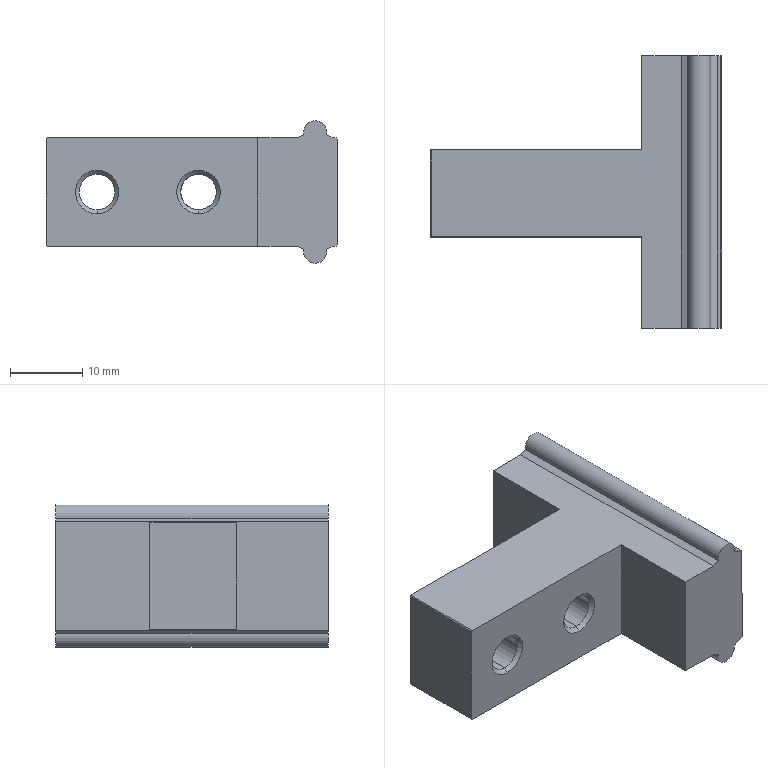Part | SolidWorks | features BaseBody 1 | 1 solid | 35 faces | box 40.2 x 37.6 x 19.68 mm | volume 11497 mm3 | plane 20 | cone 8 | cylinder 7 | commonest cylinder face diameters 4.917 x4 3.18 x3
STEP:
#1=CARTESIAN_POINT('',(-75.9,-11.,-9.84));
#2=VERTEX_POINT('',#1);
#3=CARTESIAN_POINT('',(-77.453,-11.,-7.911));
#4=VERTEX_POINT('',#3);
#5=CARTESIAN_POINT('',(-75.9,-11.,-8.25));
#6=DIRECTION('',(0.,1.,0.));
#7=DIRECTION('',(0.,0.,-1.));
#8=AXIS2_PLACEMENT_3D('',#5,#6,#7);
#9=CIRCLE('',#8,1.59);
#10=EDGE_CURVE('',#2,#4,#9,.T.);
#11=ORIENTED_EDGE('',*,*,#10,.F.);
#12=CARTESIAN_POINT('',(-75.9,-48.6,-9.84));
#13=VERTEX_POINT('',#12);
#14=CARTESIAN_POINT('',(-75.9,-48.6,-9.84));
#15=DIRECTION('',(0.,-1.,0.));
#16=VECTOR('',#15,1000.);
#17=LINE('',#14,#16);
#18=EDGE_CURVE('',#2,#13,#17,.T.);
#19=ORIENTED_EDGE('',*,*,#18,.T.);
#20=CARTESIAN_POINT('',(-77.453,-48.6,-7.911));
#21=VERTEX_POINT('',#20);
#22=CARTESIAN_POINT('',(-75.9,-48.6,-8.25));
#23=DIRECTION('',(0.,1.,0.));
#24=DIRECTION('',(0.,0.,-1.));
#25=AXIS2_PLACEMENT_3D('',#22,#23,#24);
#26=CIRCLE('',#25,1.59);
#27=EDGE_CURVE('',#13,#21,#26,.T.);
#28=ORIENTED_EDGE('',*,*,#27,.T.);
#29=CARTESIAN_POINT('',(-77.453,-48.6,-7.911));
#30=DIRECTION('',(0.,1.,0.));
#31=VECTOR('',#30,1000.);
#32=LINE('',#29,#31);
#33=EDGE_CURVE('',#21,#4,#32,.T.);
#34=ORIENTED_EDGE('',*,*,#33,.T.);
#35=EDGE_LOOP('',(#11,#19,#28,#34));
#36=FACE_OUTER_BOUND('',#35,.T.);
#37=CARTESIAN_POINT('',(-75.9,-48.6,-8.25));
#38=DIRECTION('',(0.,-1.,0.));
#39=DIRECTION('',(0.,0.,-1.));
#40=AXIS2_PLACEMENT_3D('',#37,#38,#39);
#41=CYLINDRICAL_SURFACE('',#40,1.59);
#42=ADVANCED_FACE('',(#36),#41,.T.);
#43=CARTESIAN_POINT('',(-92.,-35.459,2.458));
#44=VERTEX_POINT('',#43);
#45=CARTESIAN_POINT('',(-92.,-35.459,-2.458));
#46=VERTEX_POINT('',#45);
#47=CARTESIAN_POINT('',(-92.,-35.459,0.));
#48=DIRECTION('',(0.,-1.,0.));
#49=DIRECTION('',(0.,0.,-1.));
#50=AXIS2_PLACEMENT_3D('',#47,#48,#49);
#51=CIRCLE('',#50,2.458);
#52=EDGE_CURVE('',#44,#46,#51,.T.);
#53=ORIENTED_EDGE('',*,*,#52,.F.);
#54=CARTESIAN_POINT('',(-92.,-36.,3.));
#55=VERTEX_POINT('',#54);
#56=CARTESIAN_POINT('',(-92.,-36.,3.));
#57=DIRECTION('',(0.,-0.7071,0.7071));
#58=VECTOR('',#57,1000.);
#59=LINE('',#56,#58);
#60=EDGE_CURVE('',#44,#55,#59,.T.);
#61=ORIENTED_EDGE('',*,*,#60,.T.);
#62=CARTESIAN_POINT('',(-92.,-36.,-3.));
#63=VERTEX_POINT('',#62);
#64=CARTESIAN_POINT('',(-92.,-36.,0.));
#65=DIRECTION('',(0.,-1.,0.));
#66=DIRECTION('',(0.,0.,-1.));
#67=AXIS2_PLACEMENT_3D('',#64,#65,#66);
#68=CIRCLE('',#67,3.);
#69=EDGE_CURVE('',#55,#63,#68,.T.);
#70=ORIENTED_EDGE('',*,*,#69,.T.);
#71=CARTESIAN_POINT('',(-92.,-36.,-3.));
#72=DIRECTION('',(0.,-0.7071,-0.7071));
#73=VECTOR('',#72,1000.);
#74=LINE('',#71,#73);
#75=EDGE_CURVE('',#46,#63,#74,.T.);
#76=ORIENTED_EDGE('',*,*,#75,.F.);
#77=EDGE_LOOP('',(#53,#61,#70,#76));
#78=FACE_OUTER_BOUND('',#77,.T.);
#79=CARTESIAN_POINT('',(-92.,-36.,0.));
#80=DIRECTION('',(0.,-1.,0.));
#81=DIRECTION('',(0.,0.,-1.));
#82=AXIS2_PLACEMENT_3D('',#79,#80,#81);
#83=CONICAL_SURFACE('',#82,3.,0.7854);
#84=ADVANCED_FACE('',(#78),#83,.F.);
#85=CARTESIAN_POINT('',(-106.,-35.459,2.458));
#86=VERTEX_POINT('',#85);
#87=CARTESIAN_POINT('',(-106.,-35.459,-2.458));
#88=VERTEX_POINT('',#87);
#89=CARTESIAN_POINT('',(-106.,-35.459,0.));
#90=DIRECTION('',(0.,-1.,0.));
#91=DIRECTION('',(0.,0.,-1.));
#92=AXIS2_PLACEMENT_3D('',#89,#90,#91);
#93=CIRCLE('',#92,2.458);
#94=EDGE_CURVE('',#86,#88,#93,.T.);
#95=ORIENTED_EDGE('',*,*,#94,.F.);
#96=CARTESIAN_POINT('',(-106.,-36.,3.));
#97=VERTEX_POINT('',#96);
#98=CARTESIAN_POINT('',(-106.,-36.,3.));
#99=DIRECTION('',(0.,-0.7071,0.7071));
#100=VECTOR('',#99,1000.);
#101=LINE('',#98,#100);
#102=EDGE_CURVE('',#86,#97,#101,.T.);
#103=ORIENTED_EDGE('',*,*,#102,.T.);
#104=CARTESIAN_POINT('',(-106.,-36.,-3.));
#105=VERTEX_POINT('',#104);
#106=CARTESIAN_POINT('',(-106.,-36.,0.));
#107=DIRECTION('',(0.,-1.,0.));
#108=DIRECTION('',(0.,0.,-1.));
#109=AXIS2_PLACEMENT_3D('',#106,#107,#108);
#110=CIRCLE('',#109,3.);
#111=EDGE_CURVE('',#97,#105,#110,.T.);
#112=ORIENTED_EDGE('',*,*,#111,.T.);
#113=CARTESIAN_POINT('',(-106.,-36.,-3.));
#114=DIRECTION('',(0.,-0.7071,-0.7071));
#115=VECTOR('',#114,1000.);
#116=LINE('',#113,#115);
#117=EDGE_CURVE('',#88,#105,#116,.T.);
#118=ORIENTED_EDGE('',*,*,#117,.F.);
#119=EDGE_LOOP('',(#95,#103,#112,#118));
#120=FACE_OUTER_BOUND('',#119,.T.);
#121=CARTESIAN_POINT('',(-106.,-36.,0.));
#122=DIRECTION('',(0.,-1.,0.));
#123=DIRECTION('',(0.,0.,-1.));
#124=AXIS2_PLACEMENT_3D('',#121,#122,#123);
#125=CONICAL_SURFACE('',#124,3.,0.7854);
#126=ADVANCED_FACE('',(#120),#125,.F.);
#127=CARTESIAN_POINT('',(-89.542,-24.531,0.));
#128=VERTEX_POINT('',#127);
#129=CARTESIAN_POINT('',(-92.,-24.531,-2.458));
#130=VERTEX_POINT('',#129);
#131=CARTESIAN_POINT('',(-92.,-24.531,0.));
#132=DIRECTION('',(0.,1.,0.));
#133=DIRECTION('',(0.,0.,1.));
#134=AXIS2_PLACEMENT_3D('',#131,#132,#133);
#135=CIRCLE('',#134,2.458);
#136=EDGE_CURVE('',#128,#130,#135,.T.);
#137=ORIENTED_EDGE('',*,*,#136,.F.);
#138=CARTESIAN_POINT('',(-89.01,-24.,0.));
#139=VERTEX_POINT('',#138);
#140=CARTESIAN_POINT('',(-89.01,-24.,0.));
#141=DIRECTION('',(0.7071,0.7071,0.));
#142=VECTOR('',#141,1000.);
#143=LINE('',#140,#142);
#144=EDGE_CURVE('',#128,#139,#143,.T.);
#145=ORIENTED_EDGE('',*,*,#144,.T.);
#146=CARTESIAN_POINT('',(-94.99,-24.,0.));
#147=VERTEX_POINT('',#146);
#148=CARTESIAN_POINT('',(-92.,-24.,0.));
#149=DIRECTION('',(0.,-1.,0.));
#150=DIRECTION('',(-1.,0.,0.));
#151=AXIS2_PLACEMENT_3D('',#148,#149,#150);
#152=CIRCLE('',#151,2.99);
#153=EDGE_CURVE('',#147,#139,#152,.T.);
#154=ORIENTED_EDGE('',*,*,#153,.F.);
#155=CARTESIAN_POINT('',(-94.458,-24.531,0.));
#156=VERTEX_POINT('',#155);
#157=CARTESIAN_POINT('',(-94.99,-24.,0.));
#158=DIRECTION('',(-0.7071,0.7071,0.));
#159=VECTOR('',#158,1000.);
#160=LINE('',#157,#159);
#161=EDGE_CURVE('',#156,#147,#160,.T.);
#162=ORIENTED_EDGE('',*,*,#161,.F.);
#163=CARTESIAN_POINT('',(-92.,-24.531,0.));
#164=DIRECTION('',(0.,1.,0.));
#165=DIRECTION('',(0.,0.,1.));
#166=AXIS2_PLACEMENT_3D('',#163,#164,#165);
#167=CIRCLE('',#166,2.458);
#168=EDGE_CURVE('',#130,#156,#167,.T.);
#169=ORIENTED_EDGE('',*,*,#168,.F.);
#170=EDGE_LOOP('',(#137,#145,#154,#162,#169));
#171=FACE_OUTER_BOUND('',#170,.T.);
#172=CARTESIAN_POINT('',(-92.,-24.,0.));
#173=DIRECTION('',(0.,1.,0.));
#174=DIRECTION('',(-1.,0.,0.));
#175=AXIS2_PLACEMENT_3D('',#172,#173,#174);
#176=CONICAL_SURFACE('',#175,2.99,0.7854);
#177=ADVANCED_FACE('',(#171),#176,.F.);
#178=CARTESIAN_POINT('',(-106.,-24.532,-2.458));
#179=VERTEX_POINT('',#178);
#180=CARTESIAN_POINT('',(-106.,-24.532,2.458));
#181=VERTEX_POINT('',#180);
#182=CARTESIAN_POINT('',(-106.,-24.532,0.));
#183=DIRECTION('',(0.,1.,0.));
#184=DIRECTION('',(0.,0.,1.));
#185=AXIS2_PLACEMENT_3D('',#182,#183,#184);
#186=CIRCLE('',#185,2.458);
#187=EDGE_CURVE('',#179,#181,#186,.T.);
#188=ORIENTED_EDGE('',*,*,#187,.F.);
#189=CARTESIAN_POINT('',(-106.,-24.,-2.99));
#190=VERTEX_POINT('',#189);
#191=CARTESIAN_POINT('',(-106.,-24.,-2.99));
#192=DIRECTION('',(0.,0.7071,-0.7071));
#193=VECTOR('',#192,1000.);
#194=LINE('',#191,#193);
#195=EDGE_CURVE('',#179,#190,#194,.T.);
#196=ORIENTED_EDGE('',*,*,#195,.T.);
#197=CARTESIAN_POINT('',(-106.,-24.,2.99));
#198=VERTEX_POINT('',#197);
#199=CARTESIAN_POINT('',(-106.,-24.,0.));
#200=DIRECTION('',(0.,-1.,0.));
#201=DIRECTION('',(0.,0.,1.));
#202=AXIS2_PLACEMENT_3D('',#199,#200,#201);
#203=CIRCLE('',#202,2.99);
#204=EDGE_CURVE('',#198,#190,#203,.T.);
#205=ORIENTED_EDGE('',*,*,#204,.F.);
#206=CARTESIAN_POINT('',(-106.,-24.,2.99));
#207=DIRECTION('',(0.,0.7071,0.7071));
#208=VECTOR('',#207,1000.);
#209=LINE('',#206,#208);
#210=EDGE_CURVE('',#181,#198,#209,.T.);
#211=ORIENTED_EDGE('',*,*,#210,.F.);
#212=EDGE_LOOP('',(#188,#196,#205,#211));
#213=FACE_OUTER_BOUND('',#212,.T.);
#214=CARTESIAN_POINT('',(-106.,-24.,0.));
#215=DIRECTION('',(0.,1.,0.));
#216=DIRECTION('',(0.,0.,1.));
#217=AXIS2_PLACEMENT_3D('',#214,#215,#216);
#218=CONICAL_SURFACE('',#217,2.99,0.7854);
#219=ADVANCED_FACE('',(#213),#218,.F.);
#220=ORIENTED_EDGE('',*,*,#168,.T.);
#221=CARTESIAN_POINT('',(-92.,-24.531,2.458));
#222=VERTEX_POINT('',#221);
#223=CARTESIAN_POINT('',(-92.,-24.531,0.));
#224=DIRECTION('',(0.,1.,0.));
#225=DIRECTION('',(0.,0.,1.));
#226=AXIS2_PLACEMENT_3D('',#223,#224,#225);
#227=CIRCLE('',#226,2.458);
#228=EDGE_CURVE('',#156,#222,#227,.T.);
#229=ORIENTED_EDGE('',*,*,#228,.T.);
#230=CARTESIAN_POINT('',(-92.,-23.99,2.459));
#231=DIRECTION('',(0.,-1.,0.));
#232=VECTOR('',#231,1000.);
#233=LINE('',#230,#232);
#234=EDGE_CURVE('',#222,#44,#233,.T.);
#235=ORIENTED_EDGE('',*,*,#234,.T.);
#236=ORIENTED_EDGE('',*,*,#52,.T.);
#237=CARTESIAN_POINT('',(-92.,-23.99,-2.459));
#238=DIRECTION('',(0.,-1.,0.));
#239=VECTOR('',#238,1000.);
#240=LINE('',#237,#239);
#241=EDGE_CURVE('',#130,#46,#240,.T.);
#242=ORIENTED_EDGE('',*,*,#241,.F.);
#243=EDGE_LOOP('',(#220,#229,#235,#236,#242));
#244=FACE_OUTER_BOUND('',#243,.T.);
#245=CARTESIAN_POINT('',(-92.,-23.99,0.));
#246=DIRECTION('',(0.,-1.,0.));
#247=DIRECTION('',(0.,0.,-1.));
#248=AXIS2_PLACEMENT_3D('',#245,#246,#247);
#249=CYLINDRICAL_SURFACE('',#248,2.459);
#250=ADVANCED_FACE('',(#244),#249,.F.);
#251=ORIENTED_EDGE('',*,*,#187,.T.);
#252=CARTESIAN_POINT('',(-106.,-23.99,2.458));
#253=DIRECTION('',(0.,-1.,0.));
#254=VECTOR('',#253,1000.);
#255=LINE('',#252,#254);
#256=EDGE_CURVE('',#181,#86,#255,.T.);
#257=ORIENTED_EDGE('',*,*,#256,.T.);
#258=ORIENTED_EDGE('',*,*,#94,.T.);
#259=CARTESIAN_POINT('',(-106.,-23.99,-2.458));
#260=DIRECTION('',(0.,-1.,0.));
#261=VECTOR('',#260,1000.);
#262=LINE('',#259,#261);
#263=EDGE_CURVE('',#179,#88,#262,.T.);
#264=ORIENTED_EDGE('',*,*,#263,.F.);
#265=EDGE_LOOP('',(#251,#257,#258,#264));
#266=FACE_OUTER_BOUND('',#265,.T.);
#267=CARTESIAN_POINT('',(-106.,-23.99,0.));
#268=DIRECTION('',(0.,-1.,0.));
#269=DIRECTION('',(0.,0.,-1.));
#270=AXIS2_PLACEMENT_3D('',#267,#268,#269);
#271=CYLINDRICAL_SURFACE('',#270,2.458);
#272=ADVANCED_FACE('',(#266),#271,.F.);
#273=CARTESIAN_POINT('',(-83.8,-48.6,7.5));
#274=VERTEX_POINT('',#273);
#275=CARTESIAN_POINT('',(-78.39,-48.6,7.5));
#276=VERTEX_POINT('',#275);
#277=CARTESIAN_POINT('',(-83.8,-48.6,7.5));
#278=DIRECTION('',(1.,0.,0.));
#279=VECTOR('',#278,1000.);
#280=LINE('',#277,#279);
#281=EDGE_CURVE('',#274,#276,#280,.T.);
#282=ORIENTED_EDGE('',*,*,#281,.T.);
#283=CARTESIAN_POINT('',(-78.39,-11.,7.5));
#284=VERTEX_POINT('',#283);
#285=CARTESIAN_POINT('',(-78.39,-48.6,7.5));
#286=DIRECTION('',(0.,1.,0.));
#287=VECTOR('',#286,1000.);
#288=LINE('',#285,#287);
#289=EDGE_CURVE('',#276,#284,#288,.T.);
#290=ORIENTED_EDGE('',*,*,#289,.T.);
#291=CARTESIAN_POINT('',(-83.8,-11.,7.5));
#292=VERTEX_POINT('',#291);
#293=CARTESIAN_POINT('',(-83.8,-11.,7.5));
#294=DIRECTION('',(-1.,0.,0.));
#295=VECTOR('',#294,1000.);
#296=LINE('',#293,#295);
#297=EDGE_CURVE('',#284,#292,#296,.T.);
#298=ORIENTED_EDGE('',*,*,#297,.T.);
#299=CARTESIAN_POINT('',(-83.8,-24.,7.5));
#300=VERTEX_POINT('',#299);
#301=CARTESIAN_POINT('',(-83.8,-48.6,7.5));
#302=DIRECTION('',(0.,-1.,0.));
#303=VECTOR('',#302,1000.);
#304=LINE('',#301,#303);
#305=EDGE_CURVE('',#292,#300,#304,.T.);
#306=ORIENTED_EDGE('',*,*,#305,.T.);
#307=CARTESIAN_POINT('',(-112.859,-24.,7.5));
#308=VERTEX_POINT('',#307);
#309=CARTESIAN_POINT('',(-83.8,-24.,7.5));
#310=DIRECTION('',(-1.,0.,0.));
#311=VECTOR('',#310,1000.);
#312=LINE('',#309,#311);
#313=EDGE_CURVE('',#300,#308,#312,.T.);
#314=ORIENTED_EDGE('',*,*,#313,.T.);
#315=CARTESIAN_POINT('',(-112.859,-36.,7.5));
#316=VERTEX_POINT('',#315);
#317=CARTESIAN_POINT('',(-112.859,-48.6,7.5));
#318=DIRECTION('',(0.,-1.,0.));
#319=VECTOR('',#318,1000.);
#320=LINE('',#317,#319);
#321=EDGE_CURVE('',#308,#316,#320,.T.);
#322=ORIENTED_EDGE('',*,*,#321,.T.);
#323=CARTESIAN_POINT('',(-83.8,-36.,7.5));
#324=VERTEX_POINT('',#323);
#325=CARTESIAN_POINT('',(-83.8,-36.,7.5));
#326=DIRECTION('',(1.,0.,0.));
#327=VECTOR('',#326,1000.);
#328=LINE('',#325,#327);
#329=EDGE_CURVE('',#316,#324,#328,.T.);
#330=ORIENTED_EDGE('',*,*,#329,.T.);
#331=CARTESIAN_POINT('',(-83.8,-48.6,7.5));
#332=DIRECTION('',(0.,-1.,0.));
#333=VECTOR('',#332,1000.);
#334=LINE('',#331,#333);
#335=EDGE_CURVE('',#324,#274,#334,.T.);
#336=ORIENTED_EDGE('',*,*,#335,.T.);
#337=EDGE_LOOP('',(#282,#290,#298,#306,#314,#322,#330,#336));
#338=FACE_OUTER_BOUND('',#337,.T.);
#339=CARTESIAN_POINT('',(-83.8,-48.6,7.5));
#340=DIRECTION('',(0.,0.,1.));
#341=DIRECTION('',(1.,0.,0.));
#342=AXIS2_PLACEMENT_3D('',#339,#340,#341);
#343=PLANE('',#342);
#344=ADVANCED_FACE('',(#338),#343,.T.);
#345=CARTESIAN_POINT('',(-77.453,-48.6,7.911));
#346=VERTEX_POINT('',#345);
#347=CARTESIAN_POINT('',(-78.39,-48.6,7.5));
#348=DIRECTION('',(0.9158,0.,0.4016));
#349=VECTOR('',#348,1000.);
#350=LINE('',#347,#349);
#351=EDGE_CURVE('',#276,#346,#350,.T.);
#352=ORIENTED_EDGE('',*,*,#351,.T.);
#353=CARTESIAN_POINT('',(-77.453,-11.,7.911));
#354=VERTEX_POINT('',#353);
#355=CARTESIAN_POINT('',(-77.453,-48.6,7.911));
#356=DIRECTION('',(0.,1.,0.));
#357=VECTOR('',#356,1000.);
#358=LINE('',#355,#357);
#359=EDGE_CURVE('',#346,#354,#358,.T.);
#360=ORIENTED_EDGE('',*,*,#359,.T.);
#361=CARTESIAN_POINT('',(-78.39,-11.,7.5));
#362=DIRECTION('',(-0.9158,0.,-0.4016));
#363=VECTOR('',#362,1000.);
#364=LINE('',#361,#363);
#365=EDGE_CURVE('',#354,#284,#364,.T.);
#366=ORIENTED_EDGE('',*,*,#365,.T.);
#367=ORIENTED_EDGE('',*,*,#289,.F.);
#368=EDGE_LOOP('',(#352,#360,#366,#367));
#369=FACE_OUTER_BOUND('',#368,.T.);
#370=CARTESIAN_POINT('',(-78.39,-48.6,7.5));
#371=DIRECTION('',(-0.4016,0.,0.9158));
#372=DIRECTION('',(0.9158,0.,0.4016));
#373=AXIS2_PLACEMENT_3D('',#370,#371,#372);
#374=PLANE('',#373);
#375=ADVANCED_FACE('',(#369),#374,.T.);
#376=CARTESIAN_POINT('',(-78.39,-48.6,-7.5));
#377=VERTEX_POINT('',#376);
#378=CARTESIAN_POINT('',(-83.8,-48.6,-7.5));
#379=VERTEX_POINT('',#378);
#380=CARTESIAN_POINT('',(-75.9,-48.6,-7.5));
#381=DIRECTION('',(-1.,0.,0.));
#382=VECTOR('',#381,1000.);
#383=LINE('',#380,#382);
#384=EDGE_CURVE('',#377,#379,#383,.T.);
#385=ORIENTED_EDGE('',*,*,#384,.F.);
#386=CARTESIAN_POINT('',(-77.453,-48.6,-7.911));
#387=DIRECTION('',(-0.9158,0.,0.4016));
#388=VECTOR('',#387,1000.);
#389=LINE('',#386,#388);
#390=EDGE_CURVE('',#21,#377,#389,.T.);
#391=ORIENTED_EDGE('',*,*,#390,.F.);
#392=ORIENTED_EDGE('',*,*,#27,.F.);
#393=CARTESIAN_POINT('',(-74.347,-48.6,-7.911));
#394=VERTEX_POINT('',#393);
#395=CARTESIAN_POINT('',(-75.9,-48.6,-8.25));
#396=DIRECTION('',(0.,1.,0.));
#397=DIRECTION('',(0.,0.,-1.));
#398=AXIS2_PLACEMENT_3D('',#395,#396,#397);
#399=CIRCLE('',#398,1.59);
#400=EDGE_CURVE('',#394,#13,#399,.T.);
#401=ORIENTED_EDGE('',*,*,#400,.F.);
#402=CARTESIAN_POINT('',(-73.41,-48.6,-7.5));
#403=VERTEX_POINT('',#402);
#404=CARTESIAN_POINT('',(-73.41,-48.6,-7.5));
#405=DIRECTION('',(-0.9158,0.,-0.4016));
#406=VECTOR('',#405,1000.);
#407=LINE('',#404,#406);
#408=EDGE_CURVE('',#403,#394,#407,.T.);
#409=ORIENTED_EDGE('',*,*,#408,.F.);
#410=CARTESIAN_POINT('',(-73.012,-48.6,-7.5));
#411=VERTEX_POINT('',#410);
#412=CARTESIAN_POINT('',(-73.012,-48.6,-7.5));
#413=DIRECTION('',(-1.,0.,0.));
#414=VECTOR('',#413,1000.);
#415=LINE('',#412,#414);
#416=EDGE_CURVE('',#411,#403,#415,.T.);
#417=ORIENTED_EDGE('',*,*,#416,.F.);
#418=CARTESIAN_POINT('',(-72.8,-48.6,-7.288));
#419=VERTEX_POINT('',#418);
#420=CARTESIAN_POINT('',(-72.8,-48.6,-7.288));
#421=DIRECTION('',(-0.7071,0.,-0.7071));
#422=VECTOR('',#421,1000.);
#423=LINE('',#420,#422);
#424=EDGE_CURVE('',#419,#411,#423,.T.);
#425=ORIENTED_EDGE('',*,*,#424,.F.);
#426=CARTESIAN_POINT('',(-72.8,-48.6,7.288));
#427=VERTEX_POINT('',#426);
#428=CARTESIAN_POINT('',(-72.8,-48.6,8.25));
#429=DIRECTION('',(0.,0.,-1.));
#430=VECTOR('',#429,1000.);
#431=LINE('',#428,#430);
#432=EDGE_CURVE('',#427,#419,#431,.T.);
#433=ORIENTED_EDGE('',*,*,#432,.F.);
#434=CARTESIAN_POINT('',(-73.012,-48.6,7.5));
#435=VERTEX_POINT('',#434);
#436=CARTESIAN_POINT('',(-73.012,-48.6,7.5));
#437=DIRECTION('',(0.7071,0.,-0.7071));
#438=VECTOR('',#437,1000.);
#439=LINE('',#436,#438);
#440=EDGE_CURVE('',#435,#427,#439,.T.);
#441=ORIENTED_EDGE('',*,*,#440,.F.);
#442=CARTESIAN_POINT('',(-73.41,-48.6,7.5));
#443=VERTEX_POINT('',#442);
#444=CARTESIAN_POINT('',(-73.41,-48.6,7.5));
#445=DIRECTION('',(1.,0.,0.));
#446=VECTOR('',#445,1000.);
#447=LINE('',#444,#446);
#448=EDGE_CURVE('',#443,#435,#447,.T.);
#449=ORIENTED_EDGE('',*,*,#448,.F.);
#450=CARTESIAN_POINT('',(-74.347,-48.6,7.911));
#451=VERTEX_POINT('',#450);
#452=CARTESIAN_POINT('',(-74.347,-48.6,7.911));
#453=DIRECTION('',(0.9158,0.,-0.4016));
#454=VECTOR('',#453,1000.);
#455=LINE('',#452,#454);
#456=EDGE_CURVE('',#451,#443,#455,.T.);
#457=ORIENTED_EDGE('',*,*,#456,.F.);
#458=CARTESIAN_POINT('',(-75.9,-48.6,8.25));
#459=DIRECTION('',(0.,1.,0.));
#460=DIRECTION('',(0.,0.,-1.));
#461=AXIS2_PLACEMENT_3D('',#458,#459,#460);
#462=CIRCLE('',#461,1.59);
#463=EDGE_CURVE('',#346,#451,#462,.T.);
#464=ORIENTED_EDGE('',*,*,#463,.F.);
#465=ORIENTED_EDGE('',*,*,#351,.F.);
#466=ORIENTED_EDGE('',*,*,#281,.F.);
#467=CARTESIAN_POINT('',(-83.8,-48.6,8.25));
#468=DIRECTION('',(0.,0.,1.));
#469=VECTOR('',#468,1000.);
#470=LINE('',#467,#469);
#471=EDGE_CURVE('',#379,#274,#470,.T.);
#472=ORIENTED_EDGE('',*,*,#471,.F.);
#473=EDGE_LOOP('',(#385,#391,#392,#401,#409,#417,#425,#433,#441,#449,#457,#464,#465,#466,#472));
#474=FACE_OUTER_BOUND('',#473,.T.);
#475=CARTESIAN_POINT('',(-75.9,-48.6,8.25));
#476=DIRECTION('',(0.,1.,0.));
#477=DIRECTION('',(0.,0.,1.));
#478=AXIS2_PLACEMENT_3D('',#475,#476,#477);
#479=PLANE('',#478);
#480=ADVANCED_FACE('',(#474),#479,.F.);
#481=CARTESIAN_POINT('',(-83.8,-36.,-7.5));
#482=VERTEX_POINT('',#481);
#483=CARTESIAN_POINT('',(-83.8,-48.6,-7.5));
#484=DIRECTION('',(0.,-1.,0.));
#485=VECTOR('',#484,1000.);
#486=LINE('',#483,#485);
#487=EDGE_CURVE('',#482,#379,#486,.T.);
#488=ORIENTED_EDGE('',*,*,#487,.T.);
#489=ORIENTED_EDGE('',*,*,#471,.T.);
#490=ORIENTED_EDGE('',*,*,#335,.F.);
#491=CARTESIAN_POINT('',(-83.8,-36.,-7.5));
#492=DIRECTION('',(0.,0.,-1.));
#493=VECTOR('',#492,1000.);
#494=LINE('',#491,#493);
#495=EDGE_CURVE('',#324,#482,#494,.T.);
#496=ORIENTED_EDGE('',*,*,#495,.T.);
#497=EDGE_LOOP('',(#488,#489,#490,#496));
#498=FACE_OUTER_BOUND('',#497,.T.);
#499=CARTESIAN_POINT('',(-83.8,-48.6,-7.5));
#500=DIRECTION('',(-1.,0.,0.));
#501=DIRECTION('',(0.,0.,1.));
#502=AXIS2_PLACEMENT_3D('',#499,#500,#501);
#503=PLANE('',#502);
#504=ADVANCED_FACE('',(#498),#503,.T.);
#505=CARTESIAN_POINT('',(-92.,-36.,0.));
#506=DIRECTION('',(0.,-1.,0.));
#507=DIRECTION('',(0.,0.,-1.));
#508=AXIS2_PLACEMENT_3D('',#505,#506,#507);
#509=CIRCLE('',#508,3.);
#510=EDGE_CURVE('',#63,#55,#509,.T.);
#511=ORIENTED_EDGE('',*,*,#510,.F.);
#512=ORIENTED_EDGE('',*,*,#69,.F.);
#513=EDGE_LOOP('',(#511,#512));
#514=FACE_BOUND('',#513,.T.);
#515=CARTESIAN_POINT('',(-112.859,-36.,-7.5));
#516=VERTEX_POINT('',#515);
#517=CARTESIAN_POINT('',(-113.,-36.,-7.359));
#518=VERTEX_POINT('',#517);
#519=CARTESIAN_POINT('',(-112.859,-36.,-7.5));
#520=DIRECTION('',(-0.7071,0.,0.7071));
#521=VECTOR('',#520,1000.);
#522=LINE('',#519,#521);
#523=EDGE_CURVE('',#516,#518,#522,.T.);
#524=ORIENTED_EDGE('',*,*,#523,.F.);
#525=CARTESIAN_POINT('',(0.,-36.,-7.5));
#526=DIRECTION('',(-1.,0.,0.));
#527=VECTOR('',#526,1000.);
#528=LINE('',#525,#527);
#529=EDGE_CURVE('',#482,#516,#528,.T.);
#530=ORIENTED_EDGE('',*,*,#529,.F.);
#531=ORIENTED_EDGE('',*,*,#495,.F.);
#532=ORIENTED_EDGE('',*,*,#329,.F.);
#533=CARTESIAN_POINT('',(-113.,-36.,7.359));
#534=VERTEX_POINT('',#533);
#535=CARTESIAN_POINT('',(-113.,-36.,7.359));
#536=DIRECTION('',(0.7071,0.,0.7071));
#537=VECTOR('',#536,1000.);
#538=LINE('',#535,#537);
#539=EDGE_CURVE('',#534,#316,#538,.T.);
#540=ORIENTED_EDGE('',*,*,#539,.F.);
#541=CARTESIAN_POINT('',(-113.,-36.,0.));
#542=DIRECTION('',(0.,0.,1.));
#543=VECTOR('',#542,1000.);
#544=LINE('',#541,#543);
#545=EDGE_CURVE('',#518,#534,#544,.T.);
#546=ORIENTED_EDGE('',*,*,#545,.F.);
#547=EDGE_LOOP('',(#524,#530,#531,#532,#540,#546));
#548=FACE_OUTER_BOUND('',#547,.T.);
#549=CARTESIAN_POINT('',(-106.,-36.,0.));
#550=DIRECTION('',(0.,-1.,0.));
#551=DIRECTION('',(0.,0.,-1.));
#552=AXIS2_PLACEMENT_3D('',#549,#550,#551);
#553=CIRCLE('',#552,3.);
#554=EDGE_CURVE('',#105,#97,#553,.T.);
#555=ORIENTED_EDGE('',*,*,#554,.F.);
#556=ORIENTED_EDGE('',*,*,#111,.F.);
#557=EDGE_LOOP('',(#555,#556));
#558=FACE_BOUND('',#557,.T.);
#559=CARTESIAN_POINT('',(0.,-36.,0.));
#560=DIRECTION('',(0.,1.,0.));
#561=DIRECTION('',(0.,0.,1.));
#562=AXIS2_PLACEMENT_3D('',#559,#560,#561);
#563=PLANE('',#562);
#564=ADVANCED_FACE('',(#514,#548,#558),#563,.F.);
#565=ORIENTED_EDGE('',*,*,#539,.T.);
#566=ORIENTED_EDGE('',*,*,#321,.F.);
#567=CARTESIAN_POINT('',(-113.,-24.,7.359));
#568=VERTEX_POINT('',#567);
#569=CARTESIAN_POINT('',(-113.,-24.,7.359));
#570=DIRECTION('',(-0.7071,0.,-0.7071));
#571=VECTOR('',#570,1000.);
#572=LINE('',#569,#571);
#573=EDGE_CURVE('',#308,#568,#572,.T.);
#574=ORIENTED_EDGE('',*,*,#573,.T.);
#575=CARTESIAN_POINT('',(-113.,-36.,7.359));
#576=DIRECTION('',(0.,-1.,0.));
#577=VECTOR('',#576,1000.);
#578=LINE('',#575,#577);
#579=EDGE_CURVE('',#568,#534,#578,.T.);
#580=ORIENTED_EDGE('',*,*,#579,.T.);
#581=EDGE_LOOP('',(#565,#566,#574,#580));
#582=FACE_OUTER_BOUND('',#581,.T.);
#583=CARTESIAN_POINT('',(-113.,-36.,7.359));
#584=DIRECTION('',(-0.7071,0.,0.7071));
#585=DIRECTION('',(0.7071,0.,0.7071));
#586=AXIS2_PLACEMENT_3D('',#583,#584,#585);
#587=PLANE('',#586);
#588=ADVANCED_FACE('',(#582),#587,.T.);
#589=ORIENTED_EDGE('',*,*,#153,.T.);
#590=CARTESIAN_POINT('',(-92.,-24.,0.));
#591=DIRECTION('',(0.,-1.,0.));
#592=DIRECTION('',(-1.,0.,0.));
#593=AXIS2_PLACEMENT_3D('',#590,#591,#592);
#594=CIRCLE('',#593,2.99);
#595=EDGE_CURVE('',#139,#147,#594,.T.);
#596=ORIENTED_EDGE('',*,*,#595,.T.);
#597=EDGE_LOOP('',(#589,#596));
#598=FACE_BOUND('',#597,.T.);
#599=CARTESIAN_POINT('',(-83.8,-24.,-7.5));
#600=VERTEX_POINT('',#599);
#601=CARTESIAN_POINT('',(-112.859,-24.,-7.5));
#602=VERTEX_POINT('',#601);
#603=CARTESIAN_POINT('',(0.,-24.,-7.5));
#604=DIRECTION('',(-1.,0.,0.));
#605=VECTOR('',#604,1000.);
#606=LINE('',#603,#605);
#607=EDGE_CURVE('',#600,#602,#606,.T.);
#608=ORIENTED_EDGE('',*,*,#607,.T.);
#609=CARTESIAN_POINT('',(-113.,-24.,-7.359));
#610=VERTEX_POINT('',#609);
#611=CARTESIAN_POINT('',(-112.859,-24.,-7.5));
#612=DIRECTION('',(0.7071,0.,-0.7071));
#613=VECTOR('',#612,1000.);
#614=LINE('',#611,#613);
#615=EDGE_CURVE('',#610,#602,#614,.T.);
#616=ORIENTED_EDGE('',*,*,#615,.F.);
#617=CARTESIAN_POINT('',(-113.,-24.,0.));
#618=DIRECTION('',(0.,0.,1.));
#619=VECTOR('',#618,1000.);
#620=LINE('',#617,#619);
#621=EDGE_CURVE('',#610,#568,#620,.T.);
#622=ORIENTED_EDGE('',*,*,#621,.T.);
#623=ORIENTED_EDGE('',*,*,#573,.F.);
#624=ORIENTED_EDGE('',*,*,#313,.F.);
#625=CARTESIAN_POINT('',(-83.8,-24.,0.));
#626=DIRECTION('',(0.,0.,-1.));
#627=VECTOR('',#626,1000.);
#628=LINE('',#625,#627);
#629=EDGE_CURVE('',#300,#600,#628,.T.);
#630=ORIENTED_EDGE('',*,*,#629,.T.);
#631=EDGE_LOOP('',(#608,#616,#622,#623,#624,#630));
#632=FACE_OUTER_BOUND('',#631,.T.);
#633=ORIENTED_EDGE('',*,*,#204,.T.);
#634=CARTESIAN_POINT('',(-106.,-24.,0.));
#635=DIRECTION('',(0.,-1.,0.));
#636=DIRECTION('',(0.,0.,1.));
#637=AXIS2_PLACEMENT_3D('',#634,#635,#636);
#638=CIRCLE('',#637,2.99);
#639=EDGE_CURVE('',#190,#198,#638,.T.);
#640=ORIENTED_EDGE('',*,*,#639,.T.);
#641=EDGE_LOOP('',(#633,#640));
#642=FACE_BOUND('',#641,.T.);
#643=CARTESIAN_POINT('',(0.,-24.,0.));
#644=DIRECTION('',(0.,1.,0.));
#645=DIRECTION('',(0.,0.,1.));
#646=AXIS2_PLACEMENT_3D('',#643,#644,#645);
#647=PLANE('',#646);
#648=ADVANCED_FACE('',(#598,#632,#642),#647,.T.);
#649=CARTESIAN_POINT('',(-83.8,-11.,-7.5));
#650=VERTEX_POINT('',#649);
#651=CARTESIAN_POINT('',(-83.8,-11.,-7.5));
#652=DIRECTION('',(0.,0.,-1.));
#653=VECTOR('',#652,1000.);
#654=LINE('',#651,#653);
#655=EDGE_CURVE('',#292,#650,#654,.T.);
#656=ORIENTED_EDGE('',*,*,#655,.T.);
#657=CARTESIAN_POINT('',(-83.8,-48.6,-7.5));
#658=DIRECTION('',(0.,-1.,0.));
#659=VECTOR('',#658,1000.);
#660=LINE('',#657,#659);
#661=EDGE_CURVE('',#650,#600,#660,.T.);
#662=ORIENTED_EDGE('',*,*,#661,.T.);
#663=ORIENTED_EDGE('',*,*,#629,.F.);
#664=ORIENTED_EDGE('',*,*,#305,.F.);
#665=EDGE_LOOP('',(#656,#662,#663,#664));
#666=FACE_OUTER_BOUND('',#665,.T.);
#667=CARTESIAN_POINT('',(-83.8,-48.6,-7.5));
#668=DIRECTION('',(-1.,0.,0.));
#669=DIRECTION('',(0.,0.,1.));
#670=AXIS2_PLACEMENT_3D('',#667,#668,#669);
#671=PLANE('',#670);
#672=ADVANCED_FACE('',(#666),#671,.T.);
#673=CARTESIAN_POINT('',(-78.39,-11.,-7.5));
#674=VERTEX_POINT('',#673);
#675=CARTESIAN_POINT('',(-77.453,-11.,-7.911));
#676=DIRECTION('',(0.9158,0.,-0.4016));
#677=VECTOR('',#676,1000.);
#678=LINE('',#675,#677);
#679=EDGE_CURVE('',#674,#4,#678,.T.);
#680=ORIENTED_EDGE('',*,*,#679,.F.);
#681=CARTESIAN_POINT('',(-75.9,-11.,-7.5));
#682=DIRECTION('',(-1.,0.,0.));
#683=VECTOR('',#682,1000.);
#684=LINE('',#681,#683);
#685=EDGE_CURVE('',#674,#650,#684,.T.);
#686=ORIENTED_EDGE('',*,*,#685,.T.);
#687=ORIENTED_EDGE('',*,*,#655,.F.);
#688=ORIENTED_EDGE('',*,*,#297,.F.);
#689=ORIENTED_EDGE('',*,*,#365,.F.);
#690=CARTESIAN_POINT('',(-74.347,-11.,7.911));
#691=VERTEX_POINT('',#690);
#692=CARTESIAN_POINT('',(-75.9,-11.,8.25));
#693=DIRECTION('',(0.,1.,0.));
#694=DIRECTION('',(0.,0.,-1.));
#695=AXIS2_PLACEMENT_3D('',#692,#693,#694);
#696=CIRCLE('',#695,1.59);
#697=EDGE_CURVE('',#354,#691,#696,.T.);
#698=ORIENTED_EDGE('',*,*,#697,.T.);
#699=CARTESIAN_POINT('',(-73.41,-11.,7.5));
#700=VERTEX_POINT('',#699);
#701=CARTESIAN_POINT('',(-74.347,-11.,7.911));
#702=DIRECTION('',(-0.9158,0.,0.4016));
#703=VECTOR('',#702,1000.);
#704=LINE('',#701,#703);
#705=EDGE_CURVE('',#700,#691,#704,.T.);
#706=ORIENTED_EDGE('',*,*,#705,.F.);
#707=CARTESIAN_POINT('',(-73.012,-11.,7.5));
#708=VERTEX_POINT('',#707);
#709=CARTESIAN_POINT('',(-73.41,-11.,7.5));
#710=DIRECTION('',(-1.,0.,0.));
#711=VECTOR('',#710,1000.);
#712=LINE('',#709,#711);
#713=EDGE_CURVE('',#708,#700,#712,.T.);
#714=ORIENTED_EDGE('',*,*,#713,.F.);
#715=CARTESIAN_POINT('',(-72.8,-11.,7.288));
#716=VERTEX_POINT('',#715);
#717=CARTESIAN_POINT('',(-73.012,-11.,7.5));
#718=DIRECTION('',(-0.7071,0.,0.7071));
#719=VECTOR('',#718,1000.);
#720=LINE('',#717,#719);
#721=EDGE_CURVE('',#716,#708,#720,.T.);
#722=ORIENTED_EDGE('',*,*,#721,.F.);
#723=CARTESIAN_POINT('',(-72.8,-11.,-7.288));
#724=VERTEX_POINT('',#723);
#725=CARTESIAN_POINT('',(-72.8,-11.,8.25));
#726=DIRECTION('',(0.,0.,-1.));
#727=VECTOR('',#726,1000.);
#728=LINE('',#725,#727);
#729=EDGE_CURVE('',#716,#724,#728,.T.);
#730=ORIENTED_EDGE('',*,*,#729,.T.);
#731=CARTESIAN_POINT('',(-73.012,-11.,-7.5));
#732=VERTEX_POINT('',#731);
#733=CARTESIAN_POINT('',(-72.8,-11.,-7.288));
#734=DIRECTION('',(0.7071,0.,0.7071));
#735=VECTOR('',#734,1000.);
#736=LINE('',#733,#735);
#737=EDGE_CURVE('',#732,#724,#736,.T.);
#738=ORIENTED_EDGE('',*,*,#737,.F.);
#739=CARTESIAN_POINT('',(-73.41,-11.,-7.5));
#740=VERTEX_POINT('',#739);
#741=CARTESIAN_POINT('',(-73.012,-11.,-7.5));
#742=DIRECTION('',(1.,0.,0.));
#743=VECTOR('',#742,1000.);
#744=LINE('',#741,#743);
#745=EDGE_CURVE('',#740,#732,#744,.T.);
#746=ORIENTED_EDGE('',*,*,#745,.F.);
#747=CARTESIAN_POINT('',(-74.347,-11.,-7.911));
#748=VERTEX_POINT('',#747);
#749=CARTESIAN_POINT('',(-73.41,-11.,-7.5));
#750=DIRECTION('',(0.9158,0.,0.4016));
#751=VECTOR('',#750,1000.);
#752=LINE('',#749,#751);
#753=EDGE_CURVE('',#748,#740,#752,.T.);
#754=ORIENTED_EDGE('',*,*,#753,.F.);
#755=CARTESIAN_POINT('',(-75.9,-11.,-8.25));
#756=DIRECTION('',(0.,1.,0.));
#757=DIRECTION('',(0.,0.,-1.));
#758=AXIS2_PLACEMENT_3D('',#755,#756,#757);
#759=CIRCLE('',#758,1.59);
#760=EDGE_CURVE('',#748,#2,#759,.T.);
#761=ORIENTED_EDGE('',*,*,#760,.T.);
#762=ORIENTED_EDGE('',*,*,#10,.T.);
#763=EDGE_LOOP('',(#680,#686,#687,#688,#689,#698,#706,#714,#722,#730,#738,#746,#754,#761,#762));
#764=FACE_OUTER_BOUND('',#763,.T.);
#765=CARTESIAN_POINT('',(-75.9,-11.,8.25));
#766=DIRECTION('',(0.,1.,0.));
#767=DIRECTION('',(0.,0.,1.));
#768=AXIS2_PLACEMENT_3D('',#765,#766,#767);
#769=PLANE('',#768);
#770=ADVANCED_FACE('',(#764),#769,.T.);
#771=ORIENTED_EDGE('',*,*,#463,.T.);
#772=CARTESIAN_POINT('',(-74.347,-48.6,7.911));
#773=DIRECTION('',(0.,1.,0.));
#774=VECTOR('',#773,1000.);
#775=LINE('',#772,#774);
#776=EDGE_CURVE('',#451,#691,#775,.T.);
#777=ORIENTED_EDGE('',*,*,#776,.T.);
#778=ORIENTED_EDGE('',*,*,#697,.F.);
#779=ORIENTED_EDGE('',*,*,#359,.F.);
#780=EDGE_LOOP('',(#771,#777,#778,#779));
#781=FACE_OUTER_BOUND('',#780,.T.);
#782=CARTESIAN_POINT('',(-75.9,-48.6,8.25));
#783=DIRECTION('',(0.,-1.,0.));
#784=DIRECTION('',(0.,0.,-1.));
#785=AXIS2_PLACEMENT_3D('',#782,#783,#784);
#786=CYLINDRICAL_SURFACE('',#785,1.59);
#787=ADVANCED_FACE('',(#781),#786,.T.);
#788=ORIENTED_EDGE('',*,*,#607,.F.);
#789=ORIENTED_EDGE('',*,*,#661,.F.);
#790=ORIENTED_EDGE('',*,*,#685,.F.);
#791=CARTESIAN_POINT('',(-78.39,-48.6,-7.5));
#792=DIRECTION('',(0.,-1.,0.));
#793=VECTOR('',#792,1000.);
#794=LINE('',#791,#793);
#795=EDGE_CURVE('',#674,#377,#794,.T.);
#796=ORIENTED_EDGE('',*,*,#795,.T.);
#797=ORIENTED_EDGE('',*,*,#384,.T.);
#798=ORIENTED_EDGE('',*,*,#487,.F.);
#799=ORIENTED_EDGE('',*,*,#529,.T.);
#800=CARTESIAN_POINT('',(-112.859,-48.6,-7.5));
#801=DIRECTION('',(0.,1.,0.));
#802=VECTOR('',#801,1000.);
#803=LINE('',#800,#802);
#804=EDGE_CURVE('',#516,#602,#803,.T.);
#805=ORIENTED_EDGE('',*,*,#804,.T.);
#806=EDGE_LOOP('',(#788,#789,#790,#796,#797,#798,#799,#805));
#807=FACE_OUTER_BOUND('',#806,.T.);
#808=CARTESIAN_POINT('',(-78.39,-48.6,-7.5));
#809=DIRECTION('',(0.,0.,-1.));
#810=DIRECTION('',(-1.,0.,0.));
#811=AXIS2_PLACEMENT_3D('',#808,#809,#810);
#812=PLANE('',#811);
#813=ADVANCED_FACE('',(#807),#812,.T.);
#814=ORIENTED_EDGE('',*,*,#18,.F.);
#815=ORIENTED_EDGE('',*,*,#760,.F.);
#816=CARTESIAN_POINT('',(-74.347,-48.6,-7.911));
#817=DIRECTION('',(0.,-1.,0.));
#818=VECTOR('',#817,1000.);
#819=LINE('',#816,#818);
#820=EDGE_CURVE('',#748,#394,#819,.T.);
#821=ORIENTED_EDGE('',*,*,#820,.T.);
#822=ORIENTED_EDGE('',*,*,#400,.T.);
#823=EDGE_LOOP('',(#814,#815,#821,#822));
#824=FACE_OUTER_BOUND('',#823,.T.);
#825=CARTESIAN_POINT('',(-75.9,-48.6,-8.25));
#826=DIRECTION('',(0.,-1.,0.));
#827=DIRECTION('',(0.,0.,-1.));
#828=AXIS2_PLACEMENT_3D('',#825,#826,#827);
#829=CYLINDRICAL_SURFACE('',#828,1.59);
#830=ADVANCED_FACE('',(#824),#829,.T.);
#831=ORIENTED_EDGE('',*,*,#432,.T.);
#832=CARTESIAN_POINT('',(-72.8,-48.6,-7.288));
#833=DIRECTION('',(0.,1.,0.));
#834=VECTOR('',#833,1000.);
#835=LINE('',#832,#834);
#836=EDGE_CURVE('',#419,#724,#835,.T.);
#837=ORIENTED_EDGE('',*,*,#836,.T.);
#838=ORIENTED_EDGE('',*,*,#729,.F.);
#839=CARTESIAN_POINT('',(-72.8,-48.6,7.288));
#840=DIRECTION('',(0.,-1.,0.));
#841=VECTOR('',#840,1000.);
#842=LINE('',#839,#841);
#843=EDGE_CURVE('',#716,#427,#842,.T.);
#844=ORIENTED_EDGE('',*,*,#843,.T.);
#845=EDGE_LOOP('',(#831,#837,#838,#844));
#846=FACE_OUTER_BOUND('',#845,.T.);
#847=CARTESIAN_POINT('',(-72.8,-48.6,7.288));
#848=DIRECTION('',(1.,0.,0.));
#849=DIRECTION('',(0.,0.,-1.));
#850=AXIS2_PLACEMENT_3D('',#847,#848,#849);
#851=PLANE('',#850);
#852=ADVANCED_FACE('',(#846),#851,.T.);
#853=ORIENTED_EDGE('',*,*,#60,.F.);
#854=CARTESIAN_POINT('',(-92.,-35.459,0.));
#855=DIRECTION('',(0.,-1.,0.));
#856=DIRECTION('',(0.,0.,-1.));
#857=AXIS2_PLACEMENT_3D('',#854,#855,#856);
#858=CIRCLE('',#857,2.458);
#859=EDGE_CURVE('',#46,#44,#858,.T.);
#860=ORIENTED_EDGE('',*,*,#859,.F.);
#861=ORIENTED_EDGE('',*,*,#75,.T.);
#862=ORIENTED_EDGE('',*,*,#510,.T.);
#863=EDGE_LOOP('',(#853,#860,#861,#862));
#864=FACE_OUTER_BOUND('',#863,.T.);
#865=CARTESIAN_POINT('',(-92.,-36.,0.));
#866=DIRECTION('',(0.,-1.,0.));
#867=DIRECTION('',(0.,0.,-1.));
#868=AXIS2_PLACEMENT_3D('',#865,#866,#867);
#869=CONICAL_SURFACE('',#868,3.,0.7854);
#870=ADVANCED_FACE('',(#864),#869,.F.);
#871=ORIENTED_EDGE('',*,*,#545,.T.);
#872=ORIENTED_EDGE('',*,*,#579,.F.);
#873=ORIENTED_EDGE('',*,*,#621,.F.);
#874=CARTESIAN_POINT('',(-113.,-36.,-7.359));
#875=DIRECTION('',(0.,-1.,0.));
#876=VECTOR('',#875,1000.);
#877=LINE('',#874,#876);
#878=EDGE_CURVE('',#610,#518,#877,.T.);
#879=ORIENTED_EDGE('',*,*,#878,.T.);
#880=EDGE_LOOP('',(#871,#872,#873,#879));
#881=FACE_OUTER_BOUND('',#880,.T.);
#882=CARTESIAN_POINT('',(-113.,-36.,-7.359));
#883=DIRECTION('',(-1.,0.,0.));
#884=DIRECTION('',(0.,0.,1.));
#885=AXIS2_PLACEMENT_3D('',#882,#883,#884);
#886=PLANE('',#885);
#887=ADVANCED_FACE('',(#881),#886,.T.);
#888=ORIENTED_EDGE('',*,*,#102,.F.);
#889=CARTESIAN_POINT('',(-106.,-35.459,0.));
#890=DIRECTION('',(0.,-1.,0.));
#891=DIRECTION('',(0.,0.,-1.));
#892=AXIS2_PLACEMENT_3D('',#889,#890,#891);
#893=CIRCLE('',#892,2.458);
#894=EDGE_CURVE('',#88,#86,#893,.T.);
#895=ORIENTED_EDGE('',*,*,#894,.F.);
#896=ORIENTED_EDGE('',*,*,#117,.T.);
#897=ORIENTED_EDGE('',*,*,#554,.T.);
#898=EDGE_LOOP('',(#888,#895,#896,#897));
#899=FACE_OUTER_BOUND('',#898,.T.);
#900=CARTESIAN_POINT('',(-106.,-36.,0.));
#901=DIRECTION('',(0.,-1.,0.));
#902=DIRECTION('',(0.,0.,-1.));
#903=AXIS2_PLACEMENT_3D('',#900,#901,#902);
#904=CONICAL_SURFACE('',#903,3.,0.7854);
#905=ADVANCED_FACE('',(#899),#904,.F.);
#906=ORIENTED_EDGE('',*,*,#144,.F.);
#907=CARTESIAN_POINT('',(-92.,-24.531,0.));
#908=DIRECTION('',(0.,1.,0.));
#909=DIRECTION('',(0.,0.,1.));
#910=AXIS2_PLACEMENT_3D('',#907,#908,#909);
#911=CIRCLE('',#910,2.458);
#912=EDGE_CURVE('',#222,#128,#911,.T.);
#913=ORIENTED_EDGE('',*,*,#912,.F.);
#914=ORIENTED_EDGE('',*,*,#228,.F.);
#915=ORIENTED_EDGE('',*,*,#161,.T.);
#916=ORIENTED_EDGE('',*,*,#595,.F.);
#917=EDGE_LOOP('',(#906,#913,#914,#915,#916));
#918=FACE_OUTER_BOUND('',#917,.T.);
#919=CARTESIAN_POINT('',(-92.,-24.,0.));
#920=DIRECTION('',(0.,1.,0.));
#921=DIRECTION('',(-1.,0.,0.));
#922=AXIS2_PLACEMENT_3D('',#919,#920,#921);
#923=CONICAL_SURFACE('',#922,2.99,0.7854);
#924=ADVANCED_FACE('',(#918),#923,.F.);
#925=ORIENTED_EDGE('',*,*,#195,.F.);
#926=CARTESIAN_POINT('',(-106.,-24.532,0.));
#927=DIRECTION('',(0.,1.,0.));
#928=DIRECTION('',(0.,0.,1.));
#929=AXIS2_PLACEMENT_3D('',#926,#927,#928);
#930=CIRCLE('',#929,2.458);
#931=EDGE_CURVE('',#181,#179,#930,.T.);
#932=ORIENTED_EDGE('',*,*,#931,.F.);
#933=ORIENTED_EDGE('',*,*,#210,.T.);
#934=ORIENTED_EDGE('',*,*,#639,.F.);
#935=EDGE_LOOP('',(#925,#932,#933,#934));
#936=FACE_OUTER_BOUND('',#935,.T.);
#937=CARTESIAN_POINT('',(-106.,-24.,0.));
#938=DIRECTION('',(0.,1.,0.));
#939=DIRECTION('',(0.,0.,1.));
#940=AXIS2_PLACEMENT_3D('',#937,#938,#939);
#941=CONICAL_SURFACE('',#940,2.99,0.7854);
#942=ADVANCED_FACE('',(#936),#941,.F.);
#943=ORIENTED_EDGE('',*,*,#456,.T.);
#944=CARTESIAN_POINT('',(-73.41,-48.6,7.5));
#945=DIRECTION('',(0.,1.,0.));
#946=VECTOR('',#945,1000.);
#947=LINE('',#944,#946);
#948=EDGE_CURVE('',#443,#700,#947,.T.);
#949=ORIENTED_EDGE('',*,*,#948,.T.);
#950=ORIENTED_EDGE('',*,*,#705,.T.);
#951=ORIENTED_EDGE('',*,*,#776,.F.);
#952=EDGE_LOOP('',(#943,#949,#950,#951));
#953=FACE_OUTER_BOUND('',#952,.T.);
#954=CARTESIAN_POINT('',(-74.347,-48.6,7.911));
#955=DIRECTION('',(0.4016,0.,0.9158));
#956=DIRECTION('',(0.9158,0.,-0.4016));
#957=AXIS2_PLACEMENT_3D('',#954,#955,#956);
#958=PLANE('',#957);
#959=ADVANCED_FACE('',(#953),#958,.T.);
#960=ORIENTED_EDGE('',*,*,#523,.T.);
#961=ORIENTED_EDGE('',*,*,#878,.F.);
#962=ORIENTED_EDGE('',*,*,#615,.T.);
#963=ORIENTED_EDGE('',*,*,#804,.F.);
#964=EDGE_LOOP('',(#960,#961,#962,#963));
#965=FACE_OUTER_BOUND('',#964,.T.);
#966=CARTESIAN_POINT('',(-112.859,-36.,-7.5));
#967=DIRECTION('',(-0.7071,0.,-0.7071));
#968=DIRECTION('',(-0.7071,0.,0.7071));
#969=AXIS2_PLACEMENT_3D('',#966,#967,#968);
#970=PLANE('',#969);
#971=ADVANCED_FACE('',(#965),#970,.T.);
#972=ORIENTED_EDGE('',*,*,#390,.T.);
#973=ORIENTED_EDGE('',*,*,#795,.F.);
#974=ORIENTED_EDGE('',*,*,#679,.T.);
#975=ORIENTED_EDGE('',*,*,#33,.F.);
#976=EDGE_LOOP('',(#972,#973,#974,#975));
#977=FACE_OUTER_BOUND('',#976,.T.);
#978=CARTESIAN_POINT('',(-77.453,-48.6,-7.911));
#979=DIRECTION('',(-0.4016,0.,-0.9158));
#980=DIRECTION('',(-0.9158,0.,0.4016));
#981=AXIS2_PLACEMENT_3D('',#978,#979,#980);
#982=PLANE('',#981);
#983=ADVANCED_FACE('',(#977),#982,.T.);
#984=ORIENTED_EDGE('',*,*,#408,.T.);
#985=ORIENTED_EDGE('',*,*,#820,.F.);
#986=ORIENTED_EDGE('',*,*,#753,.T.);
#987=CARTESIAN_POINT('',(-73.41,-48.6,-7.5));
#988=DIRECTION('',(0.,-1.,0.));
#989=VECTOR('',#988,1000.);
#990=LINE('',#987,#989);
#991=EDGE_CURVE('',#740,#403,#990,.T.);
#992=ORIENTED_EDGE('',*,*,#991,.T.);
#993=EDGE_LOOP('',(#984,#985,#986,#992));
#994=FACE_OUTER_BOUND('',#993,.T.);
#995=CARTESIAN_POINT('',(-73.41,-48.6,-7.5));
#996=DIRECTION('',(0.4016,0.,-0.9158));
#997=DIRECTION('',(-0.9158,0.,-0.4016));
#998=AXIS2_PLACEMENT_3D('',#995,#996,#997);
#999=PLANE('',#998);
#1000=ADVANCED_FACE('',(#994),#999,.T.);
#1001=ORIENTED_EDGE('',*,*,#424,.T.);
#1002=CARTESIAN_POINT('',(-73.012,-48.6,-7.5));
#1003=DIRECTION('',(0.,1.,0.));
#1004=VECTOR('',#1003,1000.);
#1005=LINE('',#1002,#1004);
#1006=EDGE_CURVE('',#411,#732,#1005,.T.);
#1007=ORIENTED_EDGE('',*,*,#1006,.T.);
#1008=ORIENTED_EDGE('',*,*,#737,.T.);
#1009=ORIENTED_EDGE('',*,*,#836,.F.);
#1010=EDGE_LOOP('',(#1001,#1007,#1008,#1009));
#1011=FACE_OUTER_BOUND('',#1010,.T.);
#1012=CARTESIAN_POINT('',(-72.8,-48.6,-7.288));
#1013=DIRECTION('',(0.7071,0.,-0.7071));
#1014=DIRECTION('',(-0.7071,0.,-0.7071));
#1015=AXIS2_PLACEMENT_3D('',#1012,#1013,#1014);
#1016=PLANE('',#1015);
#1017=ADVANCED_FACE('',(#1011),#1016,.T.);
#1018=ORIENTED_EDGE('',*,*,#440,.T.);
#1019=ORIENTED_EDGE('',*,*,#843,.F.);
#1020=ORIENTED_EDGE('',*,*,#721,.T.);
#1021=CARTESIAN_POINT('',(-73.012,-48.6,7.5));
#1022=DIRECTION('',(0.,-1.,0.));
#1023=VECTOR('',#1022,1000.);
#1024=LINE('',#1021,#1023);
#1025=EDGE_CURVE('',#708,#435,#1024,.T.);
#1026=ORIENTED_EDGE('',*,*,#1025,.T.);
#1027=EDGE_LOOP('',(#1018,#1019,#1020,#1026));
#1028=FACE_OUTER_BOUND('',#1027,.T.);
#1029=CARTESIAN_POINT('',(-73.012,-48.6,7.5));
#1030=DIRECTION('',(0.7071,0.,0.7071));
#1031=DIRECTION('',(0.7071,0.,-0.7071));
#1032=AXIS2_PLACEMENT_3D('',#1029,#1030,#1031);
#1033=PLANE('',#1032);
#1034=ADVANCED_FACE('',(#1028),#1033,.T.);
#1035=ORIENTED_EDGE('',*,*,#234,.F.);
#1036=ORIENTED_EDGE('',*,*,#912,.T.);
#1037=ORIENTED_EDGE('',*,*,#136,.T.);
#1038=ORIENTED_EDGE('',*,*,#241,.T.);
#1039=ORIENTED_EDGE('',*,*,#859,.T.);
#1040=EDGE_LOOP('',(#1035,#1036,#1037,#1038,#1039));
#1041=FACE_OUTER_BOUND('',#1040,.T.);
#1042=CARTESIAN_POINT('',(-92.,-23.99,0.));
#1043=DIRECTION('',(0.,-1.,0.));
#1044=DIRECTION('',(0.,0.,-1.));
#1045=AXIS2_PLACEMENT_3D('',#1042,#1043,#1044);
#1046=CYLINDRICAL_SURFACE('',#1045,2.459);
#1047=ADVANCED_FACE('',(#1041),#1046,.F.);
#1048=ORIENTED_EDGE('',*,*,#256,.F.);
#1049=ORIENTED_EDGE('',*,*,#931,.T.);
#1050=ORIENTED_EDGE('',*,*,#263,.T.);
#1051=ORIENTED_EDGE('',*,*,#894,.T.);
#1052=EDGE_LOOP('',(#1048,#1049,#1050,#1051));
#1053=FACE_OUTER_BOUND('',#1052,.T.);
#1054=CARTESIAN_POINT('',(-106.,-23.99,0.));
#1055=DIRECTION('',(0.,-1.,0.));
#1056=DIRECTION('',(0.,0.,-1.));
#1057=AXIS2_PLACEMENT_3D('',#1054,#1055,#1056);
#1058=CYLINDRICAL_SURFACE('',#1057,2.458);
#1059=ADVANCED_FACE('',(#1053),#1058,.F.);
#1060=ORIENTED_EDGE('',*,*,#448,.T.);
#1061=ORIENTED_EDGE('',*,*,#1025,.F.);
#1062=ORIENTED_EDGE('',*,*,#713,.T.);
#1063=ORIENTED_EDGE('',*,*,#948,.F.);
#1064=EDGE_LOOP('',(#1060,#1061,#1062,#1063));
#1065=FACE_OUTER_BOUND('',#1064,.T.);
#1066=CARTESIAN_POINT('',(-73.41,-48.6,7.5));
#1067=DIRECTION('',(0.,0.,1.));
#1068=DIRECTION('',(1.,0.,0.));
#1069=AXIS2_PLACEMENT_3D('',#1066,#1067,#1068);
#1070=PLANE('',#1069);
#1071=ADVANCED_FACE('',(#1065),#1070,.T.);
#1072=ORIENTED_EDGE('',*,*,#416,.T.);
#1073=ORIENTED_EDGE('',*,*,#991,.F.);
#1074=ORIENTED_EDGE('',*,*,#745,.T.);
#1075=ORIENTED_EDGE('',*,*,#1006,.F.);
#1076=EDGE_LOOP('',(#1072,#1073,#1074,#1075));
#1077=FACE_OUTER_BOUND('',#1076,.T.);
#1078=CARTESIAN_POINT('',(-73.012,-48.6,-7.5));
#1079=DIRECTION('',(0.,0.,-1.));
#1080=DIRECTION('',(-1.,0.,0.));
#1081=AXIS2_PLACEMENT_3D('',#1078,#1079,#1080);
#1082=PLANE('',#1081);
#1083=ADVANCED_FACE('',(#1077),#1082,.T.);
#1084=CLOSED_SHELL('',(#42,#84,#126,#177,#219,#250,#272,#344,#375,#480,#504,#564,#588,#648,#672,#770,#787,#813,#830,#852,#870,#887,#905,#924,#942,#959,#971,#983,#1000,#1017,#1034,#1047,#1059,#1071,#1083));
#1085=MANIFOLD_SOLID_BREP('',#1084);
#1086=CARTESIAN_POINT('',(0.,0.,0.));
#1087=DIRECTION('',(0.,0.,1.));
#1088=DIRECTION('',(1.,0.,0.));
#1089=AXIS2_PLACEMENT_3D('',#1086,#1087,#1088);
#1090=(LENGTH_UNIT()NAMED_UNIT(*)SI_UNIT(.MILLI.,.METRE.));
#1091=UNCERTAINTY_MEASURE_WITH_UNIT(LENGTH_MEASURE(0.00001),#1090,'','');
#1092=(NAMED_UNIT(*)PLANE_ANGLE_UNIT()SI_UNIT($,.RADIAN.));
#1093=(NAMED_UNIT(*)SI_UNIT($,.STERADIAN.)SOLID_ANGLE_UNIT());
#1094=(GEOMETRIC_REPRESENTATION_CONTEXT(3)GLOBAL_UNCERTAINTY_ASSIGNED_CONTEXT((#1091))GLOBAL_UNIT_ASSIGNED_CONTEXT((#1090,#1092,#1093))REPRESENTATION_CONTEXT('',''));
#1095=ADVANCED_BREP_SHAPE_REPRESENTATION('',(#1085,#1089),#1094);